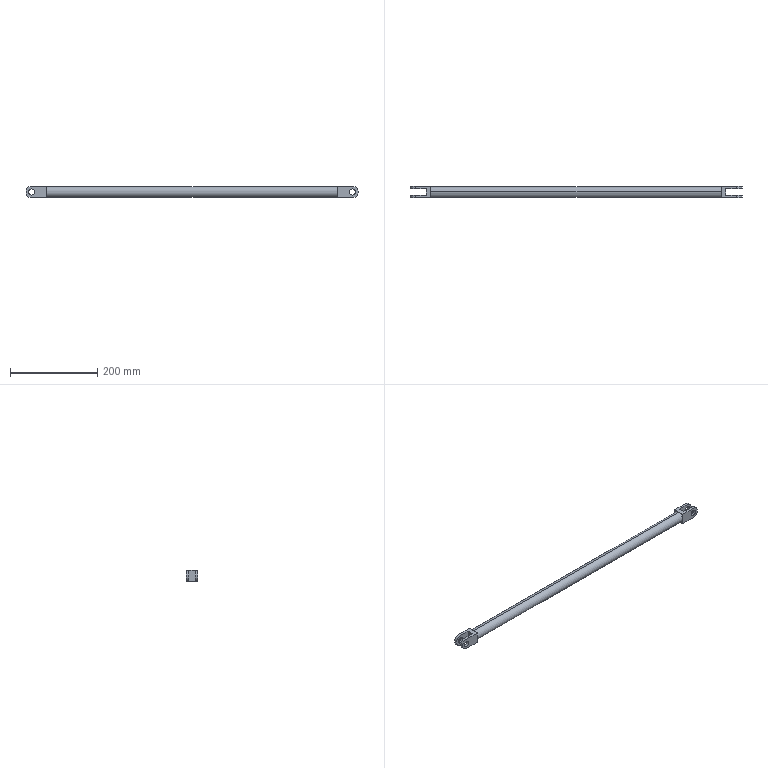Part | SolidWorks | features MirrorStock 1 | 3 solids | 34 faces | box 763 x 26 x 26 mm | volume 170096 mm3 | plane 18 | cylinder 16 | commonest cylinder face diameters 14 x8 26 x4 19 x2 25 x2
STEP:
#1=CARTESIAN_POINT('',(0.,13.,-7.));
#2=VERTEX_POINT('',#1);
#3=CARTESIAN_POINT('',(0.,13.,7.));
#4=VERTEX_POINT('',#3);
#5=CARTESIAN_POINT('',(0.,13.,0.));
#6=DIRECTION('',(0.,-1.,0.));
#7=DIRECTION('',(0.,0.,-1.));
#8=AXIS2_PLACEMENT_3D('',#5,#6,#7);
#9=CIRCLE('',#8,7.);
#10=EDGE_CURVE('',#2,#4,#9,.T.);
#11=ORIENTED_EDGE('',*,*,#10,.F.);
#12=CARTESIAN_POINT('',(0.,7.,-7.));
#13=VERTEX_POINT('',#12);
#14=CARTESIAN_POINT('',(0.,13.,-7.));
#15=DIRECTION('',(0.,-1.,0.));
#16=VECTOR('',#15,1000.);
#17=LINE('',#14,#16);
#18=EDGE_CURVE('',#2,#13,#17,.T.);
#19=ORIENTED_EDGE('',*,*,#18,.T.);
#20=CARTESIAN_POINT('',(0.,7.,7.));
#21=VERTEX_POINT('',#20);
#22=CARTESIAN_POINT('',(0.,7.,0.));
#23=DIRECTION('',(0.,-1.,0.));
#24=DIRECTION('',(-1.,0.,0.));
#25=AXIS2_PLACEMENT_3D('',#22,#23,#24);
#26=CIRCLE('',#25,7.);
#27=EDGE_CURVE('',#13,#21,#26,.T.);
#28=ORIENTED_EDGE('',*,*,#27,.T.);
#29=CARTESIAN_POINT('',(0.,13.,7.));
#30=DIRECTION('',(0.,-1.,0.));
#31=VECTOR('',#30,1000.);
#32=LINE('',#29,#31);
#33=EDGE_CURVE('',#4,#21,#32,.T.);
#34=ORIENTED_EDGE('',*,*,#33,.F.);
#35=EDGE_LOOP('',(#11,#19,#28,#34));
#36=FACE_OUTER_BOUND('',#35,.T.);
#37=CARTESIAN_POINT('',(0.,13.,0.));
#38=DIRECTION('',(0.,-1.,0.));
#39=DIRECTION('',(0.,0.,1.));
#40=AXIS2_PLACEMENT_3D('',#37,#38,#39);
#41=CYLINDRICAL_SURFACE('',#40,7.);
#42=ADVANCED_FACE('',(#36),#41,.F.);
#43=CARTESIAN_POINT('',(0.,-7.,7.));
#44=VERTEX_POINT('',#43);
#45=CARTESIAN_POINT('',(0.,-7.,-7.));
#46=VERTEX_POINT('',#45);
#47=CARTESIAN_POINT('',(0.,-7.,0.));
#48=DIRECTION('',(0.,1.,0.));
#49=DIRECTION('',(1.,0.,0.));
#50=AXIS2_PLACEMENT_3D('',#47,#48,#49);
#51=CIRCLE('',#50,7.);
#52=EDGE_CURVE('',#44,#46,#51,.T.);
#53=ORIENTED_EDGE('',*,*,#52,.T.);
#54=CARTESIAN_POINT('',(0.,-13.,-7.));
#55=VERTEX_POINT('',#54);
#56=CARTESIAN_POINT('',(0.,13.,-7.));
#57=DIRECTION('',(0.,-1.,0.));
#58=VECTOR('',#57,1000.);
#59=LINE('',#56,#58);
#60=EDGE_CURVE('',#46,#55,#59,.T.);
#61=ORIENTED_EDGE('',*,*,#60,.T.);
#62=CARTESIAN_POINT('',(0.,-13.,7.));
#63=VERTEX_POINT('',#62);
#64=CARTESIAN_POINT('',(0.,-13.,0.));
#65=DIRECTION('',(0.,-1.,0.));
#66=DIRECTION('',(0.,0.,-1.));
#67=AXIS2_PLACEMENT_3D('',#64,#65,#66);
#68=CIRCLE('',#67,7.);
#69=EDGE_CURVE('',#55,#63,#68,.T.);
#70=ORIENTED_EDGE('',*,*,#69,.T.);
#71=CARTESIAN_POINT('',(0.,13.,7.));
#72=DIRECTION('',(0.,-1.,0.));
#73=VECTOR('',#72,1000.);
#74=LINE('',#71,#73);
#75=EDGE_CURVE('',#44,#63,#74,.T.);
#76=ORIENTED_EDGE('',*,*,#75,.F.);
#77=EDGE_LOOP('',(#53,#61,#70,#76));
#78=FACE_OUTER_BOUND('',#77,.T.);
#79=CARTESIAN_POINT('',(0.,13.,0.));
#80=DIRECTION('',(0.,-1.,0.));
#81=DIRECTION('',(0.,0.,1.));
#82=AXIS2_PLACEMENT_3D('',#79,#80,#81);
#83=CYLINDRICAL_SURFACE('',#82,7.);
#84=ADVANCED_FACE('',(#78),#83,.F.);
#85=CARTESIAN_POINT('',(0.,-7.,-13.));
#86=VERTEX_POINT('',#85);
#87=CARTESIAN_POINT('',(0.,-13.,-13.));
#88=VERTEX_POINT('',#87);
#89=CARTESIAN_POINT('',(0.,13.,-13.));
#90=DIRECTION('',(0.,-1.,0.));
#91=VECTOR('',#90,1000.);
#92=LINE('',#89,#91);
#93=EDGE_CURVE('',#86,#88,#92,.T.);
#94=ORIENTED_EDGE('',*,*,#93,.T.);
#95=CARTESIAN_POINT('',(0.,-13.,13.));
#96=VERTEX_POINT('',#95);
#97=CARTESIAN_POINT('',(0.,-13.,0.));
#98=DIRECTION('',(0.,-1.,0.));
#99=DIRECTION('',(0.,0.,-1.));
#100=AXIS2_PLACEMENT_3D('',#97,#98,#99);
#101=CIRCLE('',#100,13.);
#102=EDGE_CURVE('',#96,#88,#101,.T.);
#103=ORIENTED_EDGE('',*,*,#102,.F.);
#104=CARTESIAN_POINT('',(0.,-7.,13.));
#105=VERTEX_POINT('',#104);
#106=CARTESIAN_POINT('',(0.,13.,13.));
#107=DIRECTION('',(0.,-1.,0.));
#108=VECTOR('',#107,1000.);
#109=LINE('',#106,#108);
#110=EDGE_CURVE('',#105,#96,#109,.T.);
#111=ORIENTED_EDGE('',*,*,#110,.F.);
#112=CARTESIAN_POINT('',(0.,-7.,0.));
#113=DIRECTION('',(0.,1.,0.));
#114=DIRECTION('',(1.,0.,0.));
#115=AXIS2_PLACEMENT_3D('',#112,#113,#114);
#116=CIRCLE('',#115,13.);
#117=EDGE_CURVE('',#86,#105,#116,.T.);
#118=ORIENTED_EDGE('',*,*,#117,.F.);
#119=EDGE_LOOP('',(#94,#103,#111,#118));
#120=FACE_OUTER_BOUND('',#119,.T.);
#121=CARTESIAN_POINT('',(0.,13.,0.));
#122=DIRECTION('',(0.,-1.,0.));
#123=DIRECTION('',(0.,0.,1.));
#124=AXIS2_PLACEMENT_3D('',#121,#122,#123);
#125=CYLINDRICAL_SURFACE('',#124,13.);
#126=ADVANCED_FACE('',(#120),#125,.T.);
#127=ORIENTED_EDGE('',*,*,#60,.F.);
#128=CARTESIAN_POINT('',(0.,-7.,0.));
#129=DIRECTION('',(0.,1.,0.));
#130=DIRECTION('',(1.,0.,0.));
#131=AXIS2_PLACEMENT_3D('',#128,#129,#130);
#132=CIRCLE('',#131,7.);
#133=EDGE_CURVE('',#46,#44,#132,.T.);
#134=ORIENTED_EDGE('',*,*,#133,.T.);
#135=ORIENTED_EDGE('',*,*,#75,.T.);
#136=CARTESIAN_POINT('',(0.,-13.,0.));
#137=DIRECTION('',(0.,-1.,0.));
#138=DIRECTION('',(0.,0.,-1.));
#139=AXIS2_PLACEMENT_3D('',#136,#137,#138);
#140=CIRCLE('',#139,7.);
#141=EDGE_CURVE('',#63,#55,#140,.T.);
#142=ORIENTED_EDGE('',*,*,#141,.T.);
#143=EDGE_LOOP('',(#127,#134,#135,#142));
#144=FACE_OUTER_BOUND('',#143,.T.);
#145=CARTESIAN_POINT('',(0.,13.,0.));
#146=DIRECTION('',(0.,-1.,0.));
#147=DIRECTION('',(0.,0.,1.));
#148=AXIS2_PLACEMENT_3D('',#145,#146,#147);
#149=CYLINDRICAL_SURFACE('',#148,7.);
#150=ADVANCED_FACE('',(#144),#149,.F.);
#151=CARTESIAN_POINT('',(0.,13.,13.));
#152=VERTEX_POINT('',#151);
#153=CARTESIAN_POINT('',(0.,13.,-13.));
#154=VERTEX_POINT('',#153);
#155=CARTESIAN_POINT('',(0.,13.,0.));
#156=DIRECTION('',(0.,-1.,0.));
#157=DIRECTION('',(0.,0.,-1.));
#158=AXIS2_PLACEMENT_3D('',#155,#156,#157);
#159=CIRCLE('',#158,13.);
#160=EDGE_CURVE('',#152,#154,#159,.T.);
#161=ORIENTED_EDGE('',*,*,#160,.F.);
#162=CARTESIAN_POINT('',(35.,13.,13.));
#163=VERTEX_POINT('',#162);
#164=CARTESIAN_POINT('',(0.,13.,13.));
#165=DIRECTION('',(-1.,0.,0.));
#166=VECTOR('',#165,1000.);
#167=LINE('',#164,#166);
#168=EDGE_CURVE('',#163,#152,#167,.T.);
#169=ORIENTED_EDGE('',*,*,#168,.F.);
#170=CARTESIAN_POINT('',(35.,13.,-13.));
#171=VERTEX_POINT('',#170);
#172=CARTESIAN_POINT('',(35.,13.,13.));
#173=DIRECTION('',(0.,0.,1.));
#174=VECTOR('',#173,1000.);
#175=LINE('',#172,#174);
#176=EDGE_CURVE('',#171,#163,#175,.T.);
#177=ORIENTED_EDGE('',*,*,#176,.F.);
#178=CARTESIAN_POINT('',(0.,13.,-13.));
#179=DIRECTION('',(1.,0.,0.));
#180=VECTOR('',#179,1000.);
#181=LINE('',#178,#180);
#182=EDGE_CURVE('',#154,#171,#181,.T.);
#183=ORIENTED_EDGE('',*,*,#182,.F.);
#184=EDGE_LOOP('',(#161,#169,#177,#183));
#185=FACE_OUTER_BOUND('',#184,.T.);
#186=CARTESIAN_POINT('',(0.,13.,0.));
#187=DIRECTION('',(0.,-1.,0.));
#188=DIRECTION('',(0.,0.,-1.));
#189=AXIS2_PLACEMENT_3D('',#186,#187,#188);
#190=CIRCLE('',#189,7.);
#191=EDGE_CURVE('',#4,#2,#190,.T.);
#192=ORIENTED_EDGE('',*,*,#191,.T.);
#193=ORIENTED_EDGE('',*,*,#10,.T.);
#194=EDGE_LOOP('',(#192,#193));
#195=FACE_BOUND('',#194,.T.);
#196=CARTESIAN_POINT('',(0.,13.,0.));
#197=DIRECTION('',(0.,1.,0.));
#198=DIRECTION('',(0.,0.,-1.));
#199=AXIS2_PLACEMENT_3D('',#196,#197,#198);
#200=PLANE('',#199);
#201=ADVANCED_FACE('',(#185,#195),#200,.T.);
#202=ORIENTED_EDGE('',*,*,#102,.T.);
#203=CARTESIAN_POINT('',(35.,-13.,-13.));
#204=VERTEX_POINT('',#203);
#205=CARTESIAN_POINT('',(0.,-13.,-13.));
#206=DIRECTION('',(1.,0.,0.));
#207=VECTOR('',#206,1000.);
#208=LINE('',#205,#207);
#209=EDGE_CURVE('',#88,#204,#208,.T.);
#210=ORIENTED_EDGE('',*,*,#209,.T.);
#211=CARTESIAN_POINT('',(35.,-13.,13.));
#212=VERTEX_POINT('',#211);
#213=CARTESIAN_POINT('',(35.,-13.,13.));
#214=DIRECTION('',(0.,0.,1.));
#215=VECTOR('',#214,1000.);
#216=LINE('',#213,#215);
#217=EDGE_CURVE('',#204,#212,#216,.T.);
#218=ORIENTED_EDGE('',*,*,#217,.T.);
#219=CARTESIAN_POINT('',(0.,-13.,13.));
#220=DIRECTION('',(-1.,0.,0.));
#221=VECTOR('',#220,1000.);
#222=LINE('',#219,#221);
#223=EDGE_CURVE('',#212,#96,#222,.T.);
#224=ORIENTED_EDGE('',*,*,#223,.T.);
#225=EDGE_LOOP('',(#202,#210,#218,#224));
#226=FACE_OUTER_BOUND('',#225,.T.);
#227=ORIENTED_EDGE('',*,*,#141,.F.);
#228=ORIENTED_EDGE('',*,*,#69,.F.);
#229=EDGE_LOOP('',(#227,#228));
#230=FACE_BOUND('',#229,.T.);
#231=CARTESIAN_POINT('',(0.,-13.,0.));
#232=DIRECTION('',(0.,1.,0.));
#233=DIRECTION('',(0.,0.,-1.));
#234=AXIS2_PLACEMENT_3D('',#231,#232,#233);
#235=PLANE('',#234);
#236=ADVANCED_FACE('',(#226,#230),#235,.F.);
#237=CARTESIAN_POINT('',(0.,7.,13.));
#238=VERTEX_POINT('',#237);
#239=CARTESIAN_POINT('',(0.,13.,13.));
#240=DIRECTION('',(0.,-1.,0.));
#241=VECTOR('',#240,1000.);
#242=LINE('',#239,#241);
#243=EDGE_CURVE('',#152,#238,#242,.T.);
#244=ORIENTED_EDGE('',*,*,#243,.F.);
#245=ORIENTED_EDGE('',*,*,#160,.T.);
#246=CARTESIAN_POINT('',(0.,7.,-13.));
#247=VERTEX_POINT('',#246);
#248=CARTESIAN_POINT('',(0.,13.,-13.));
#249=DIRECTION('',(0.,-1.,0.));
#250=VECTOR('',#249,1000.);
#251=LINE('',#248,#250);
#252=EDGE_CURVE('',#154,#247,#251,.T.);
#253=ORIENTED_EDGE('',*,*,#252,.T.);
#254=CARTESIAN_POINT('',(0.,7.,0.));
#255=DIRECTION('',(0.,-1.,0.));
#256=DIRECTION('',(-1.,0.,0.));
#257=AXIS2_PLACEMENT_3D('',#254,#255,#256);
#258=CIRCLE('',#257,13.);
#259=EDGE_CURVE('',#238,#247,#258,.T.);
#260=ORIENTED_EDGE('',*,*,#259,.F.);
#261=EDGE_LOOP('',(#244,#245,#253,#260));
#262=FACE_OUTER_BOUND('',#261,.T.);
#263=CARTESIAN_POINT('',(0.,13.,0.));
#264=DIRECTION('',(0.,-1.,0.));
#265=DIRECTION('',(0.,0.,1.));
#266=AXIS2_PLACEMENT_3D('',#263,#264,#265);
#267=CYLINDRICAL_SURFACE('',#266,13.);
#268=ADVANCED_FACE('',(#262),#267,.T.);
#269=CARTESIAN_POINT('',(25.,-7.,-13.));
#270=VERTEX_POINT('',#269);
#271=CARTESIAN_POINT('',(25.,7.,-13.));
#272=VERTEX_POINT('',#271);
#273=CARTESIAN_POINT('',(25.,-7.,-13.));
#274=DIRECTION('',(0.,1.,0.));
#275=VECTOR('',#274,1000.);
#276=LINE('',#273,#275);
#277=EDGE_CURVE('',#270,#272,#276,.T.);
#278=ORIENTED_EDGE('',*,*,#277,.T.);
#279=CARTESIAN_POINT('',(-25.,7.,-13.));
#280=DIRECTION('',(-1.,0.,0.));
#281=VECTOR('',#280,1000.);
#282=LINE('',#279,#281);
#283=EDGE_CURVE('',#272,#247,#282,.T.);
#284=ORIENTED_EDGE('',*,*,#283,.T.);
#285=ORIENTED_EDGE('',*,*,#252,.F.);
#286=ORIENTED_EDGE('',*,*,#182,.T.);
#287=CARTESIAN_POINT('',(35.,13.,-13.));
#288=DIRECTION('',(0.,-1.,0.));
#289=VECTOR('',#288,1000.);
#290=LINE('',#287,#289);
#291=EDGE_CURVE('',#171,#204,#290,.T.);
#292=ORIENTED_EDGE('',*,*,#291,.T.);
#293=ORIENTED_EDGE('',*,*,#209,.F.);
#294=ORIENTED_EDGE('',*,*,#93,.F.);
#295=CARTESIAN_POINT('',(-25.,-7.,-13.));
#296=DIRECTION('',(1.,0.,0.));
#297=VECTOR('',#296,1000.);
#298=LINE('',#295,#297);
#299=EDGE_CURVE('',#86,#270,#298,.T.);
#300=ORIENTED_EDGE('',*,*,#299,.T.);
#301=EDGE_LOOP('',(#278,#284,#285,#286,#292,#293,#294,#300));
#302=FACE_OUTER_BOUND('',#301,.T.);
#303=CARTESIAN_POINT('',(0.,13.,-13.));
#304=DIRECTION('',(0.,0.,1.));
#305=DIRECTION('',(-1.,0.,0.));
#306=AXIS2_PLACEMENT_3D('',#303,#304,#305);
#307=PLANE('',#306);
#308=ADVANCED_FACE('',(#302),#307,.F.);
#309=ORIENTED_EDGE('',*,*,#217,.F.);
#310=ORIENTED_EDGE('',*,*,#291,.F.);
#311=ORIENTED_EDGE('',*,*,#176,.T.);
#312=CARTESIAN_POINT('',(35.,13.,13.));
#313=DIRECTION('',(0.,-1.,0.));
#314=VECTOR('',#313,1000.);
#315=LINE('',#312,#314);
#316=EDGE_CURVE('',#163,#212,#315,.T.);
#317=ORIENTED_EDGE('',*,*,#316,.T.);
#318=EDGE_LOOP('',(#309,#310,#311,#317));
#319=FACE_OUTER_BOUND('',#318,.T.);
#320=CARTESIAN_POINT('',(35.,13.,13.));
#321=DIRECTION('',(-1.,0.,0.));
#322=DIRECTION('',(0.,0.,-1.));
#323=AXIS2_PLACEMENT_3D('',#320,#321,#322);
#324=PLANE('',#323);
#325=ADVANCED_FACE('',(#319),#324,.F.);
#326=ORIENTED_EDGE('',*,*,#110,.T.);
#327=ORIENTED_EDGE('',*,*,#223,.F.);
#328=ORIENTED_EDGE('',*,*,#316,.F.);
#329=ORIENTED_EDGE('',*,*,#168,.T.);
#330=ORIENTED_EDGE('',*,*,#243,.T.);
#331=CARTESIAN_POINT('',(25.,7.,13.));
#332=VERTEX_POINT('',#331);
#333=CARTESIAN_POINT('',(-25.,7.,13.));
#334=DIRECTION('',(-1.,0.,0.));
#335=VECTOR('',#334,1000.);
#336=LINE('',#333,#335);
#337=EDGE_CURVE('',#332,#238,#336,.T.);
#338=ORIENTED_EDGE('',*,*,#337,.F.);
#339=CARTESIAN_POINT('',(25.,-7.,13.));
#340=VERTEX_POINT('',#339);
#341=CARTESIAN_POINT('',(25.,-7.,13.));
#342=DIRECTION('',(0.,1.,0.));
#343=VECTOR('',#342,1000.);
#344=LINE('',#341,#343);
#345=EDGE_CURVE('',#340,#332,#344,.T.);
#346=ORIENTED_EDGE('',*,*,#345,.F.);
#347=CARTESIAN_POINT('',(-25.,-7.,13.));
#348=DIRECTION('',(1.,0.,0.));
#349=VECTOR('',#348,1000.);
#350=LINE('',#347,#349);
#351=EDGE_CURVE('',#105,#340,#350,.T.);
#352=ORIENTED_EDGE('',*,*,#351,.F.);
#353=EDGE_LOOP('',(#326,#327,#328,#329,#330,#338,#346,#352));
#354=FACE_OUTER_BOUND('',#353,.T.);
#355=CARTESIAN_POINT('',(0.,13.,13.));
#356=DIRECTION('',(0.,0.,-1.));
#357=DIRECTION('',(1.,0.,0.));
#358=AXIS2_PLACEMENT_3D('',#355,#356,#357);
#359=PLANE('',#358);
#360=ADVANCED_FACE('',(#354),#359,.F.);
#361=ORIENTED_EDGE('',*,*,#18,.F.);
#362=ORIENTED_EDGE('',*,*,#191,.F.);
#363=ORIENTED_EDGE('',*,*,#33,.T.);
#364=CARTESIAN_POINT('',(0.,7.,0.));
#365=DIRECTION('',(0.,-1.,0.));
#366=DIRECTION('',(-1.,0.,0.));
#367=AXIS2_PLACEMENT_3D('',#364,#365,#366);
#368=CIRCLE('',#367,7.);
#369=EDGE_CURVE('',#21,#13,#368,.T.);
#370=ORIENTED_EDGE('',*,*,#369,.T.);
#371=EDGE_LOOP('',(#361,#362,#363,#370));
#372=FACE_OUTER_BOUND('',#371,.T.);
#373=CARTESIAN_POINT('',(0.,13.,0.));
#374=DIRECTION('',(0.,-1.,0.));
#375=DIRECTION('',(0.,0.,1.));
#376=AXIS2_PLACEMENT_3D('',#373,#374,#375);
#377=CYLINDRICAL_SURFACE('',#376,7.);
#378=ADVANCED_FACE('',(#372),#377,.F.);
#379=ORIENTED_EDGE('',*,*,#52,.F.);
#380=ORIENTED_EDGE('',*,*,#133,.F.);
#381=EDGE_LOOP('',(#379,#380));
#382=FACE_BOUND('',#381,.T.);
#383=ORIENTED_EDGE('',*,*,#299,.F.);
#384=ORIENTED_EDGE('',*,*,#117,.T.);
#385=ORIENTED_EDGE('',*,*,#351,.T.);
#386=CARTESIAN_POINT('',(25.,-7.,13.));
#387=DIRECTION('',(0.,0.,-1.));
#388=VECTOR('',#387,1000.);
#389=LINE('',#386,#388);
#390=EDGE_CURVE('',#340,#270,#389,.T.);
#391=ORIENTED_EDGE('',*,*,#390,.T.);
#392=EDGE_LOOP('',(#383,#384,#385,#391));
#393=FACE_OUTER_BOUND('',#392,.T.);
#394=CARTESIAN_POINT('',(-25.,-7.,13.));
#395=DIRECTION('',(0.,-1.,0.));
#396=DIRECTION('',(1.,0.,0.));
#397=AXIS2_PLACEMENT_3D('',#394,#395,#396);
#398=PLANE('',#397);
#399=ADVANCED_FACE('',(#382,#393),#398,.F.);
#400=ORIENTED_EDGE('',*,*,#369,.F.);
#401=ORIENTED_EDGE('',*,*,#27,.F.);
#402=EDGE_LOOP('',(#400,#401));
#403=FACE_BOUND('',#402,.T.);
#404=ORIENTED_EDGE('',*,*,#337,.T.);
#405=ORIENTED_EDGE('',*,*,#259,.T.);
#406=ORIENTED_EDGE('',*,*,#283,.F.);
#407=CARTESIAN_POINT('',(25.,7.,13.));
#408=DIRECTION('',(0.,0.,-1.));
#409=VECTOR('',#408,1000.);
#410=LINE('',#407,#409);
#411=EDGE_CURVE('',#332,#272,#410,.T.);
#412=ORIENTED_EDGE('',*,*,#411,.F.);
#413=EDGE_LOOP('',(#404,#405,#406,#412));
#414=FACE_OUTER_BOUND('',#413,.T.);
#415=CARTESIAN_POINT('',(-25.,7.,13.));
#416=DIRECTION('',(0.,1.,0.));
#417=DIRECTION('',(-1.,0.,0.));
#418=AXIS2_PLACEMENT_3D('',#415,#416,#417);
#419=PLANE('',#418);
#420=ADVANCED_FACE('',(#403,#414),#419,.F.);
#421=ORIENTED_EDGE('',*,*,#411,.T.);
#422=ORIENTED_EDGE('',*,*,#277,.F.);
#423=ORIENTED_EDGE('',*,*,#390,.F.);
#424=ORIENTED_EDGE('',*,*,#345,.T.);
#425=EDGE_LOOP('',(#421,#422,#423,#424));
#426=FACE_OUTER_BOUND('',#425,.T.);
#427=CARTESIAN_POINT('',(25.,-7.,13.));
#428=DIRECTION('',(1.,0.,0.));
#429=DIRECTION('',(0.,0.,1.));
#430=AXIS2_PLACEMENT_3D('',#427,#428,#429);
#431=PLANE('',#430);
#432=ADVANCED_FACE('',(#426),#431,.F.);
#433=CLOSED_SHELL('',(#42,#84,#126,#150,#201,#236,#268,#308,#325,#360,#378,#399,#420,#432));
#434=MANIFOLD_SOLID_BREP('',#433);
#435=CARTESIAN_POINT('',(702.,0.,9.5));
#436=VERTEX_POINT('',#435);
#437=CARTESIAN_POINT('',(702.,0.,-9.5));
#438=VERTEX_POINT('',#437);
#439=CARTESIAN_POINT('',(702.,0.,0.));
#440=DIRECTION('',(-1.,0.,0.));
#441=DIRECTION('',(0.,0.,1.));
#442=AXIS2_PLACEMENT_3D('',#439,#440,#441);
#443=CIRCLE('',#442,9.5);
#444=EDGE_CURVE('',#436,#438,#443,.T.);
#445=ORIENTED_EDGE('',*,*,#444,.F.);
#446=CARTESIAN_POINT('',(35.,0.,9.5));
#447=VERTEX_POINT('',#446);
#448=CARTESIAN_POINT('',(702.,0.,9.5));
#449=DIRECTION('',(-1.,0.,0.));
#450=VECTOR('',#449,1000.);
#451=LINE('',#448,#450);
#452=EDGE_CURVE('',#436,#447,#451,.T.);
#453=ORIENTED_EDGE('',*,*,#452,.T.);
#454=CARTESIAN_POINT('',(35.,0.,-9.5));
#455=VERTEX_POINT('',#454);
#456=CARTESIAN_POINT('',(35.,0.,0.));
#457=DIRECTION('',(-1.,0.,0.));
#458=DIRECTION('',(0.,0.,1.));
#459=AXIS2_PLACEMENT_3D('',#456,#457,#458);
#460=CIRCLE('',#459,9.5);
#461=EDGE_CURVE('',#447,#455,#460,.T.);
#462=ORIENTED_EDGE('',*,*,#461,.T.);
#463=CARTESIAN_POINT('',(702.,0.,-9.5));
#464=DIRECTION('',(-1.,0.,0.));
#465=VECTOR('',#464,1000.);
#466=LINE('',#463,#465);
#467=EDGE_CURVE('',#438,#455,#466,.T.);
#468=ORIENTED_EDGE('',*,*,#467,.F.);
#469=EDGE_LOOP('',(#445,#453,#462,#468));
#470=FACE_OUTER_BOUND('',#469,.T.);
#471=CARTESIAN_POINT('',(702.,0.,0.));
#472=DIRECTION('',(-1.,0.,0.));
#473=DIRECTION('',(0.,0.,-1.));
#474=AXIS2_PLACEMENT_3D('',#471,#472,#473);
#475=CYLINDRICAL_SURFACE('',#474,9.5);
#476=ADVANCED_FACE('',(#470),#475,.F.);
#477=CARTESIAN_POINT('',(702.,0.,-12.5));
#478=VERTEX_POINT('',#477);
#479=CARTESIAN_POINT('',(702.,0.,12.5));
#480=VERTEX_POINT('',#479);
#481=CARTESIAN_POINT('',(702.,0.,0.));
#482=DIRECTION('',(-1.,0.,0.));
#483=DIRECTION('',(0.,0.,1.));
#484=AXIS2_PLACEMENT_3D('',#481,#482,#483);
#485=CIRCLE('',#484,12.5);
#486=EDGE_CURVE('',#478,#480,#485,.T.);
#487=ORIENTED_EDGE('',*,*,#486,.T.);
#488=CARTESIAN_POINT('',(35.,0.,12.5));
#489=VERTEX_POINT('',#488);
#490=CARTESIAN_POINT('',(702.,0.,12.5));
#491=DIRECTION('',(-1.,0.,0.));
#492=VECTOR('',#491,1000.);
#493=LINE('',#490,#492);
#494=EDGE_CURVE('',#480,#489,#493,.T.);
#495=ORIENTED_EDGE('',*,*,#494,.T.);
#496=CARTESIAN_POINT('',(35.,0.,-12.5));
#497=VERTEX_POINT('',#496);
#498=CARTESIAN_POINT('',(35.,0.,0.));
#499=DIRECTION('',(-1.,0.,0.));
#500=DIRECTION('',(0.,0.,1.));
#501=AXIS2_PLACEMENT_3D('',#498,#499,#500);
#502=CIRCLE('',#501,12.5);
#503=EDGE_CURVE('',#497,#489,#502,.T.);
#504=ORIENTED_EDGE('',*,*,#503,.F.);
#505=CARTESIAN_POINT('',(702.,0.,-12.5));
#506=DIRECTION('',(-1.,0.,0.));
#507=VECTOR('',#506,1000.);
#508=LINE('',#505,#507);
#509=EDGE_CURVE('',#478,#497,#508,.T.);
#510=ORIENTED_EDGE('',*,*,#509,.F.);
#511=EDGE_LOOP('',(#487,#495,#504,#510));
#512=FACE_OUTER_BOUND('',#511,.T.);
#513=CARTESIAN_POINT('',(702.,0.,0.));
#514=DIRECTION('',(-1.,0.,0.));
#515=DIRECTION('',(0.,0.,-1.));
#516=AXIS2_PLACEMENT_3D('',#513,#514,#515);
#517=CYLINDRICAL_SURFACE('',#516,12.5);
#518=ADVANCED_FACE('',(#512),#517,.T.);
#519=ORIENTED_EDGE('',*,*,#486,.F.);
#520=CARTESIAN_POINT('',(702.,0.,0.));
#521=DIRECTION('',(-1.,0.,0.));
#522=DIRECTION('',(0.,0.,1.));
#523=AXIS2_PLACEMENT_3D('',#520,#521,#522);
#524=CIRCLE('',#523,12.5);
#525=EDGE_CURVE('',#480,#478,#524,.T.);
#526=ORIENTED_EDGE('',*,*,#525,.F.);
#527=EDGE_LOOP('',(#519,#526));
#528=FACE_OUTER_BOUND('',#527,.T.);
#529=CARTESIAN_POINT('',(702.,0.,0.));
#530=DIRECTION('',(-1.,0.,0.));
#531=DIRECTION('',(0.,0.,1.));
#532=AXIS2_PLACEMENT_3D('',#529,#530,#531);
#533=CIRCLE('',#532,9.5);
#534=EDGE_CURVE('',#438,#436,#533,.T.);
#535=ORIENTED_EDGE('',*,*,#534,.T.);
#536=ORIENTED_EDGE('',*,*,#444,.T.);
#537=EDGE_LOOP('',(#535,#536));
#538=FACE_BOUND('',#537,.T.);
#539=CARTESIAN_POINT('',(702.,0.,0.));
#540=DIRECTION('',(1.,0.,0.));
#541=DIRECTION('',(0.,0.,1.));
#542=AXIS2_PLACEMENT_3D('',#539,#540,#541);
#543=PLANE('',#542);
#544=ADVANCED_FACE('',(#528,#538),#543,.T.);
#545=ORIENTED_EDGE('',*,*,#503,.T.);
#546=CARTESIAN_POINT('',(35.,0.,0.));
#547=DIRECTION('',(-1.,0.,0.));
#548=DIRECTION('',(0.,0.,1.));
#549=AXIS2_PLACEMENT_3D('',#546,#547,#548);
#550=CIRCLE('',#549,12.5);
#551=EDGE_CURVE('',#489,#497,#550,.T.);
#552=ORIENTED_EDGE('',*,*,#551,.T.);
#553=EDGE_LOOP('',(#545,#552));
#554=FACE_OUTER_BOUND('',#553,.T.);
#555=CARTESIAN_POINT('',(35.,0.,0.));
#556=DIRECTION('',(-1.,0.,0.));
#557=DIRECTION('',(0.,0.,1.));
#558=AXIS2_PLACEMENT_3D('',#555,#556,#557);
#559=CIRCLE('',#558,9.5);
#560=EDGE_CURVE('',#455,#447,#559,.T.);
#561=ORIENTED_EDGE('',*,*,#560,.F.);
#562=ORIENTED_EDGE('',*,*,#461,.F.);
#563=EDGE_LOOP('',(#561,#562));
#564=FACE_BOUND('',#563,.T.);
#565=CARTESIAN_POINT('',(35.,0.,0.));
#566=DIRECTION('',(1.,0.,0.));
#567=DIRECTION('',(0.,0.,1.));
#568=AXIS2_PLACEMENT_3D('',#565,#566,#567);
#569=PLANE('',#568);
#570=ADVANCED_FACE('',(#554,#564),#569,.F.);
#571=ORIENTED_EDGE('',*,*,#494,.F.);
#572=ORIENTED_EDGE('',*,*,#525,.T.);
#573=ORIENTED_EDGE('',*,*,#509,.T.);
#574=ORIENTED_EDGE('',*,*,#551,.F.);
#575=EDGE_LOOP('',(#571,#572,#573,#574));
#576=FACE_OUTER_BOUND('',#575,.T.);
#577=CARTESIAN_POINT('',(702.,0.,0.));
#578=DIRECTION('',(-1.,0.,0.));
#579=DIRECTION('',(0.,0.,-1.));
#580=AXIS2_PLACEMENT_3D('',#577,#578,#579);
#581=CYLINDRICAL_SURFACE('',#580,12.5);
#582=ADVANCED_FACE('',(#576),#581,.T.);
#583=ORIENTED_EDGE('',*,*,#452,.F.);
#584=ORIENTED_EDGE('',*,*,#534,.F.);
#585=ORIENTED_EDGE('',*,*,#467,.T.);
#586=ORIENTED_EDGE('',*,*,#560,.T.);
#587=EDGE_LOOP('',(#583,#584,#585,#586));
#588=FACE_OUTER_BOUND('',#587,.T.);
#589=CARTESIAN_POINT('',(702.,0.,0.));
#590=DIRECTION('',(-1.,0.,0.));
#591=DIRECTION('',(0.,0.,-1.));
#592=AXIS2_PLACEMENT_3D('',#589,#590,#591);
#593=CYLINDRICAL_SURFACE('',#592,9.5);
#594=ADVANCED_FACE('',(#588),#593,.F.);
#595=CLOSED_SHELL('',(#476,#518,#544,#570,#582,#594));
#596=MANIFOLD_SOLID_BREP('',#595);
#597=CARTESIAN_POINT('',(737.,13.,7.));
#598=VERTEX_POINT('',#597);
#599=CARTESIAN_POINT('',(737.,13.,-7.));
#600=VERTEX_POINT('',#599);
#601=CARTESIAN_POINT('',(737.,13.,0.));
#602=DIRECTION('',(0.,1.,0.));
#603=DIRECTION('',(0.,0.,-1.));
#604=AXIS2_PLACEMENT_3D('',#601,#602,#603);
#605=CIRCLE('',#604,7.);
#606=EDGE_CURVE('',#598,#600,#605,.T.);
#607=ORIENTED_EDGE('',*,*,#606,.T.);
#608=CARTESIAN_POINT('',(737.,7.,-7.));
#609=VERTEX_POINT('',#608);
#610=CARTESIAN_POINT('',(737.,13.,-7.));
#611=DIRECTION('',(0.,-1.,0.));
#612=VECTOR('',#611,1000.);
#613=LINE('',#610,#612);
#614=EDGE_CURVE('',#600,#609,#613,.T.);
#615=ORIENTED_EDGE('',*,*,#614,.T.);
#616=CARTESIAN_POINT('',(737.,7.,7.));
#617=VERTEX_POINT('',#616);
#618=CARTESIAN_POINT('',(737.,7.,0.));
#619=DIRECTION('',(0.,1.,0.));
#620=DIRECTION('',(1.,0.,0.));
#621=AXIS2_PLACEMENT_3D('',#618,#619,#620);
#622=CIRCLE('',#621,7.);
#623=EDGE_CURVE('',#617,#609,#622,.T.);
#624=ORIENTED_EDGE('',*,*,#623,.F.);
#625=CARTESIAN_POINT('',(737.,13.,7.));
#626=DIRECTION('',(0.,-1.,0.));
#627=VECTOR('',#626,1000.);
#628=LINE('',#625,#627);
#629=EDGE_CURVE('',#598,#617,#628,.T.);
#630=ORIENTED_EDGE('',*,*,#629,.F.);
#631=EDGE_LOOP('',(#607,#615,#624,#630));
#632=FACE_OUTER_BOUND('',#631,.T.);
#633=CARTESIAN_POINT('',(737.,13.,0.));
#634=DIRECTION('',(0.,-1.,0.));
#635=DIRECTION('',(0.,0.,1.));
#636=AXIS2_PLACEMENT_3D('',#633,#634,#635);
#637=CYLINDRICAL_SURFACE('',#636,7.);
#638=ADVANCED_FACE('',(#632),#637,.F.);
#639=CARTESIAN_POINT('',(737.,-7.,-7.));
#640=VERTEX_POINT('',#639);
#641=CARTESIAN_POINT('',(737.,-7.,7.));
#642=VERTEX_POINT('',#641);
#643=CARTESIAN_POINT('',(737.,-7.,0.));
#644=DIRECTION('',(0.,-1.,0.));
#645=DIRECTION('',(-1.,0.,0.));
#646=AXIS2_PLACEMENT_3D('',#643,#644,#645);
#647=CIRCLE('',#646,7.);
#648=EDGE_CURVE('',#640,#642,#647,.T.);
#649=ORIENTED_EDGE('',*,*,#648,.F.);
#650=CARTESIAN_POINT('',(737.,-13.,-7.));
#651=VERTEX_POINT('',#650);
#652=CARTESIAN_POINT('',(737.,13.,-7.));
#653=DIRECTION('',(0.,-1.,0.));
#654=VECTOR('',#653,1000.);
#655=LINE('',#652,#654);
#656=EDGE_CURVE('',#640,#651,#655,.T.);
#657=ORIENTED_EDGE('',*,*,#656,.T.);
#658=CARTESIAN_POINT('',(737.,-13.,7.));
#659=VERTEX_POINT('',#658);
#660=CARTESIAN_POINT('',(737.,-13.,0.));
#661=DIRECTION('',(0.,1.,0.));
#662=DIRECTION('',(0.,0.,-1.));
#663=AXIS2_PLACEMENT_3D('',#660,#661,#662);
#664=CIRCLE('',#663,7.);
#665=EDGE_CURVE('',#659,#651,#664,.T.);
#666=ORIENTED_EDGE('',*,*,#665,.F.);
#667=CARTESIAN_POINT('',(737.,13.,7.));
#668=DIRECTION('',(0.,-1.,0.));
#669=VECTOR('',#668,1000.);
#670=LINE('',#667,#669);
#671=EDGE_CURVE('',#642,#659,#670,.T.);
#672=ORIENTED_EDGE('',*,*,#671,.F.);
#673=EDGE_LOOP('',(#649,#657,#666,#672));
#674=FACE_OUTER_BOUND('',#673,.T.);
#675=CARTESIAN_POINT('',(737.,13.,0.));
#676=DIRECTION('',(0.,-1.,0.));
#677=DIRECTION('',(0.,0.,1.));
#678=AXIS2_PLACEMENT_3D('',#675,#676,#677);
#679=CYLINDRICAL_SURFACE('',#678,7.);
#680=ADVANCED_FACE('',(#674),#679,.F.);
#681=CARTESIAN_POINT('',(737.,-7.,-13.));
#682=VERTEX_POINT('',#681);
#683=CARTESIAN_POINT('',(737.,-13.,-13.));
#684=VERTEX_POINT('',#683);
#685=CARTESIAN_POINT('',(737.,13.,-13.));
#686=DIRECTION('',(0.,-1.,0.));
#687=VECTOR('',#686,1000.);
#688=LINE('',#685,#687);
#689=EDGE_CURVE('',#682,#684,#688,.T.);
#690=ORIENTED_EDGE('',*,*,#689,.F.);
#691=CARTESIAN_POINT('',(737.,-7.,13.));
#692=VERTEX_POINT('',#691);
#693=CARTESIAN_POINT('',(737.,-7.,0.));
#694=DIRECTION('',(0.,-1.,0.));
#695=DIRECTION('',(-1.,0.,0.));
#696=AXIS2_PLACEMENT_3D('',#693,#694,#695);
#697=CIRCLE('',#696,13.);
#698=EDGE_CURVE('',#682,#692,#697,.T.);
#699=ORIENTED_EDGE('',*,*,#698,.T.);
#700=CARTESIAN_POINT('',(737.,-13.,13.));
#701=VERTEX_POINT('',#700);
#702=CARTESIAN_POINT('',(737.,13.,13.));
#703=DIRECTION('',(0.,-1.,0.));
#704=VECTOR('',#703,1000.);
#705=LINE('',#702,#704);
#706=EDGE_CURVE('',#692,#701,#705,.T.);
#707=ORIENTED_EDGE('',*,*,#706,.T.);
#708=CARTESIAN_POINT('',(737.,-13.,0.));
#709=DIRECTION('',(0.,1.,0.));
#710=DIRECTION('',(0.,0.,-1.));
#711=AXIS2_PLACEMENT_3D('',#708,#709,#710);
#712=CIRCLE('',#711,13.);
#713=EDGE_CURVE('',#701,#684,#712,.T.);
#714=ORIENTED_EDGE('',*,*,#713,.T.);
#715=EDGE_LOOP('',(#690,#699,#707,#714));
#716=FACE_OUTER_BOUND('',#715,.T.);
#717=CARTESIAN_POINT('',(737.,13.,0.));
#718=DIRECTION('',(0.,-1.,0.));
#719=DIRECTION('',(0.,0.,1.));
#720=AXIS2_PLACEMENT_3D('',#717,#718,#719);
#721=CYLINDRICAL_SURFACE('',#720,13.);
#722=ADVANCED_FACE('',(#716),#721,.T.);
#723=ORIENTED_EDGE('',*,*,#656,.F.);
#724=CARTESIAN_POINT('',(737.,-7.,0.));
#725=DIRECTION('',(0.,-1.,0.));
#726=DIRECTION('',(-1.,0.,0.));
#727=AXIS2_PLACEMENT_3D('',#724,#725,#726);
#728=CIRCLE('',#727,7.);
#729=EDGE_CURVE('',#642,#640,#728,.T.);
#730=ORIENTED_EDGE('',*,*,#729,.F.);
#731=ORIENTED_EDGE('',*,*,#671,.T.);
#732=CARTESIAN_POINT('',(737.,-13.,0.));
#733=DIRECTION('',(0.,1.,0.));
#734=DIRECTION('',(0.,0.,-1.));
#735=AXIS2_PLACEMENT_3D('',#732,#733,#734);
#736=CIRCLE('',#735,7.);
#737=EDGE_CURVE('',#651,#659,#736,.T.);
#738=ORIENTED_EDGE('',*,*,#737,.F.);
#739=EDGE_LOOP('',(#723,#730,#731,#738));
#740=FACE_OUTER_BOUND('',#739,.T.);
#741=CARTESIAN_POINT('',(737.,13.,0.));
#742=DIRECTION('',(0.,-1.,0.));
#743=DIRECTION('',(0.,0.,1.));
#744=AXIS2_PLACEMENT_3D('',#741,#742,#743);
#745=CYLINDRICAL_SURFACE('',#744,7.);
#746=ADVANCED_FACE('',(#740),#745,.F.);
#747=CARTESIAN_POINT('',(737.,13.,13.));
#748=VERTEX_POINT('',#747);
#749=CARTESIAN_POINT('',(737.,13.,-13.));
#750=VERTEX_POINT('',#749);
#751=CARTESIAN_POINT('',(737.,13.,0.));
#752=DIRECTION('',(0.,1.,0.));
#753=DIRECTION('',(0.,0.,-1.));
#754=AXIS2_PLACEMENT_3D('',#751,#752,#753);
#755=CIRCLE('',#754,13.);
#756=EDGE_CURVE('',#748,#750,#755,.T.);
#757=ORIENTED_EDGE('',*,*,#756,.T.);
#758=CARTESIAN_POINT('',(702.,13.,-13.));
#759=VERTEX_POINT('',#758);
#760=CARTESIAN_POINT('',(737.,13.,-13.));
#761=DIRECTION('',(-1.,0.,0.));
#762=VECTOR('',#761,1000.);
#763=LINE('',#760,#762);
#764=EDGE_CURVE('',#750,#759,#763,.T.);
#765=ORIENTED_EDGE('',*,*,#764,.T.);
#766=CARTESIAN_POINT('',(702.,13.,13.));
#767=VERTEX_POINT('',#766);
#768=CARTESIAN_POINT('',(702.,13.,13.));
#769=DIRECTION('',(0.,0.,1.));
#770=VECTOR('',#769,1000.);
#771=LINE('',#768,#770);
#772=EDGE_CURVE('',#759,#767,#771,.T.);
#773=ORIENTED_EDGE('',*,*,#772,.T.);
#774=CARTESIAN_POINT('',(737.,13.,13.));
#775=DIRECTION('',(1.,0.,0.));
#776=VECTOR('',#775,1000.);
#777=LINE('',#774,#776);
#778=EDGE_CURVE('',#767,#748,#777,.T.);
#779=ORIENTED_EDGE('',*,*,#778,.T.);
#780=EDGE_LOOP('',(#757,#765,#773,#779));
#781=FACE_OUTER_BOUND('',#780,.T.);
#782=ORIENTED_EDGE('',*,*,#606,.F.);
#783=CARTESIAN_POINT('',(737.,13.,0.));
#784=DIRECTION('',(0.,1.,0.));
#785=DIRECTION('',(0.,0.,-1.));
#786=AXIS2_PLACEMENT_3D('',#783,#784,#785);
#787=CIRCLE('',#786,7.);
#788=EDGE_CURVE('',#600,#598,#787,.T.);
#789=ORIENTED_EDGE('',*,*,#788,.F.);
#790=EDGE_LOOP('',(#782,#789));
#791=FACE_BOUND('',#790,.T.);
#792=CARTESIAN_POINT('',(737.,13.,0.));
#793=DIRECTION('',(0.,1.,0.));
#794=DIRECTION('',(0.,0.,-1.));
#795=AXIS2_PLACEMENT_3D('',#792,#793,#794);
#796=PLANE('',#795);
#797=ADVANCED_FACE('',(#781,#791),#796,.T.);
#798=ORIENTED_EDGE('',*,*,#713,.F.);
#799=CARTESIAN_POINT('',(702.,-13.,13.));
#800=VERTEX_POINT('',#799);
#801=CARTESIAN_POINT('',(737.,-13.,13.));
#802=DIRECTION('',(1.,0.,0.));
#803=VECTOR('',#802,1000.);
#804=LINE('',#801,#803);
#805=EDGE_CURVE('',#800,#701,#804,.T.);
#806=ORIENTED_EDGE('',*,*,#805,.F.);
#807=CARTESIAN_POINT('',(702.,-13.,-13.));
#808=VERTEX_POINT('',#807);
#809=CARTESIAN_POINT('',(702.,-13.,13.));
#810=DIRECTION('',(0.,0.,1.));
#811=VECTOR('',#810,1000.);
#812=LINE('',#809,#811);
#813=EDGE_CURVE('',#808,#800,#812,.T.);
#814=ORIENTED_EDGE('',*,*,#813,.F.);
#815=CARTESIAN_POINT('',(737.,-13.,-13.));
#816=DIRECTION('',(-1.,0.,0.));
#817=VECTOR('',#816,1000.);
#818=LINE('',#815,#817);
#819=EDGE_CURVE('',#684,#808,#818,.T.);
#820=ORIENTED_EDGE('',*,*,#819,.F.);
#821=EDGE_LOOP('',(#798,#806,#814,#820));
#822=FACE_OUTER_BOUND('',#821,.T.);
#823=ORIENTED_EDGE('',*,*,#665,.T.);
#824=ORIENTED_EDGE('',*,*,#737,.T.);
#825=EDGE_LOOP('',(#823,#824));
#826=FACE_BOUND('',#825,.T.);
#827=CARTESIAN_POINT('',(737.,-13.,0.));
#828=DIRECTION('',(0.,1.,0.));
#829=DIRECTION('',(0.,0.,-1.));
#830=AXIS2_PLACEMENT_3D('',#827,#828,#829);
#831=PLANE('',#830);
#832=ADVANCED_FACE('',(#822,#826),#831,.F.);
#833=CARTESIAN_POINT('',(737.,7.,13.));
#834=VERTEX_POINT('',#833);
#835=CARTESIAN_POINT('',(737.,13.,13.));
#836=DIRECTION('',(0.,-1.,0.));
#837=VECTOR('',#836,1000.);
#838=LINE('',#835,#837);
#839=EDGE_CURVE('',#748,#834,#838,.T.);
#840=ORIENTED_EDGE('',*,*,#839,.T.);
#841=CARTESIAN_POINT('',(737.,7.,-13.));
#842=VERTEX_POINT('',#841);
#843=CARTESIAN_POINT('',(737.,7.,0.));
#844=DIRECTION('',(0.,1.,0.));
#845=DIRECTION('',(1.,0.,0.));
#846=AXIS2_PLACEMENT_3D('',#843,#844,#845);
#847=CIRCLE('',#846,13.);
#848=EDGE_CURVE('',#834,#842,#847,.T.);
#849=ORIENTED_EDGE('',*,*,#848,.T.);
#850=CARTESIAN_POINT('',(737.,13.,-13.));
#851=DIRECTION('',(0.,-1.,0.));
#852=VECTOR('',#851,1000.);
#853=LINE('',#850,#852);
#854=EDGE_CURVE('',#750,#842,#853,.T.);
#855=ORIENTED_EDGE('',*,*,#854,.F.);
#856=ORIENTED_EDGE('',*,*,#756,.F.);
#857=EDGE_LOOP('',(#840,#849,#855,#856));
#858=FACE_OUTER_BOUND('',#857,.T.);
#859=CARTESIAN_POINT('',(737.,13.,0.));
#860=DIRECTION('',(0.,-1.,0.));
#861=DIRECTION('',(0.,0.,1.));
#862=AXIS2_PLACEMENT_3D('',#859,#860,#861);
#863=CYLINDRICAL_SURFACE('',#862,13.);
#864=ADVANCED_FACE('',(#858),#863,.T.);
#865=CARTESIAN_POINT('',(712.,-7.,-13.));
#866=VERTEX_POINT('',#865);
#867=CARTESIAN_POINT('',(712.,7.,-13.));
#868=VERTEX_POINT('',#867);
#869=CARTESIAN_POINT('',(712.,-7.,-13.));
#870=DIRECTION('',(0.,1.,0.));
#871=VECTOR('',#870,1000.);
#872=LINE('',#869,#871);
#873=EDGE_CURVE('',#866,#868,#872,.T.);
#874=ORIENTED_EDGE('',*,*,#873,.F.);
#875=CARTESIAN_POINT('',(762.,-7.,-13.));
#876=DIRECTION('',(-1.,0.,0.));
#877=VECTOR('',#876,1000.);
#878=LINE('',#875,#877);
#879=EDGE_CURVE('',#682,#866,#878,.T.);
#880=ORIENTED_EDGE('',*,*,#879,.F.);
#881=ORIENTED_EDGE('',*,*,#689,.T.);
#882=ORIENTED_EDGE('',*,*,#819,.T.);
#883=CARTESIAN_POINT('',(702.,13.,-13.));
#884=DIRECTION('',(0.,-1.,0.));
#885=VECTOR('',#884,1000.);
#886=LINE('',#883,#885);
#887=EDGE_CURVE('',#759,#808,#886,.T.);
#888=ORIENTED_EDGE('',*,*,#887,.F.);
#889=ORIENTED_EDGE('',*,*,#764,.F.);
#890=ORIENTED_EDGE('',*,*,#854,.T.);
#891=CARTESIAN_POINT('',(762.,7.,-13.));
#892=DIRECTION('',(1.,0.,0.));
#893=VECTOR('',#892,1000.);
#894=LINE('',#891,#893);
#895=EDGE_CURVE('',#868,#842,#894,.T.);
#896=ORIENTED_EDGE('',*,*,#895,.F.);
#897=EDGE_LOOP('',(#874,#880,#881,#882,#888,#889,#890,#896));
#898=FACE_OUTER_BOUND('',#897,.T.);
#899=CARTESIAN_POINT('',(737.,13.,-13.));
#900=DIRECTION('',(0.,0.,1.));
#901=DIRECTION('',(1.,0.,0.));
#902=AXIS2_PLACEMENT_3D('',#899,#900,#901);
#903=PLANE('',#902);
#904=ADVANCED_FACE('',(#898),#903,.F.);
#905=ORIENTED_EDGE('',*,*,#813,.T.);
#906=CARTESIAN_POINT('',(702.,13.,13.));
#907=DIRECTION('',(0.,-1.,0.));
#908=VECTOR('',#907,1000.);
#909=LINE('',#906,#908);
#910=EDGE_CURVE('',#767,#800,#909,.T.);
#911=ORIENTED_EDGE('',*,*,#910,.F.);
#912=ORIENTED_EDGE('',*,*,#772,.F.);
#913=ORIENTED_EDGE('',*,*,#887,.T.);
#914=EDGE_LOOP('',(#905,#911,#912,#913));
#915=FACE_OUTER_BOUND('',#914,.T.);
#916=CARTESIAN_POINT('',(702.,13.,13.));
#917=DIRECTION('',(1.,0.,0.));
#918=DIRECTION('',(0.,0.,-1.));
#919=AXIS2_PLACEMENT_3D('',#916,#917,#918);
#920=PLANE('',#919);
#921=ADVANCED_FACE('',(#915),#920,.F.);
#922=ORIENTED_EDGE('',*,*,#706,.F.);
#923=CARTESIAN_POINT('',(712.,-7.,13.));
#924=VERTEX_POINT('',#923);
#925=CARTESIAN_POINT('',(762.,-7.,13.));
#926=DIRECTION('',(-1.,0.,0.));
#927=VECTOR('',#926,1000.);
#928=LINE('',#925,#927);
#929=EDGE_CURVE('',#692,#924,#928,.T.);
#930=ORIENTED_EDGE('',*,*,#929,.T.);
#931=CARTESIAN_POINT('',(712.,7.,13.));
#932=VERTEX_POINT('',#931);
#933=CARTESIAN_POINT('',(712.,-7.,13.));
#934=DIRECTION('',(0.,1.,0.));
#935=VECTOR('',#934,1000.);
#936=LINE('',#933,#935);
#937=EDGE_CURVE('',#924,#932,#936,.T.);
#938=ORIENTED_EDGE('',*,*,#937,.T.);
#939=CARTESIAN_POINT('',(762.,7.,13.));
#940=DIRECTION('',(1.,0.,0.));
#941=VECTOR('',#940,1000.);
#942=LINE('',#939,#941);
#943=EDGE_CURVE('',#932,#834,#942,.T.);
#944=ORIENTED_EDGE('',*,*,#943,.T.);
#945=ORIENTED_EDGE('',*,*,#839,.F.);
#946=ORIENTED_EDGE('',*,*,#778,.F.);
#947=ORIENTED_EDGE('',*,*,#910,.T.);
#948=ORIENTED_EDGE('',*,*,#805,.T.);
#949=EDGE_LOOP('',(#922,#930,#938,#944,#945,#946,#947,#948));
#950=FACE_OUTER_BOUND('',#949,.T.);
#951=CARTESIAN_POINT('',(737.,13.,13.));
#952=DIRECTION('',(0.,0.,-1.));
#953=DIRECTION('',(-1.,0.,0.));
#954=AXIS2_PLACEMENT_3D('',#951,#952,#953);
#955=PLANE('',#954);
#956=ADVANCED_FACE('',(#950),#955,.F.);
#957=ORIENTED_EDGE('',*,*,#614,.F.);
#958=ORIENTED_EDGE('',*,*,#788,.T.);
#959=ORIENTED_EDGE('',*,*,#629,.T.);
#960=CARTESIAN_POINT('',(737.,7.,0.));
#961=DIRECTION('',(0.,1.,0.));
#962=DIRECTION('',(1.,0.,0.));
#963=AXIS2_PLACEMENT_3D('',#960,#961,#962);
#964=CIRCLE('',#963,7.);
#965=EDGE_CURVE('',#609,#617,#964,.T.);
#966=ORIENTED_EDGE('',*,*,#965,.F.);
#967=EDGE_LOOP('',(#957,#958,#959,#966));
#968=FACE_OUTER_BOUND('',#967,.T.);
#969=CARTESIAN_POINT('',(737.,13.,0.));
#970=DIRECTION('',(0.,-1.,0.));
#971=DIRECTION('',(0.,0.,1.));
#972=AXIS2_PLACEMENT_3D('',#969,#970,#971);
#973=CYLINDRICAL_SURFACE('',#972,7.);
#974=ADVANCED_FACE('',(#968),#973,.F.);
#975=ORIENTED_EDGE('',*,*,#729,.T.);
#976=ORIENTED_EDGE('',*,*,#648,.T.);
#977=EDGE_LOOP('',(#975,#976));
#978=FACE_BOUND('',#977,.T.);
#979=ORIENTED_EDGE('',*,*,#879,.T.);
#980=CARTESIAN_POINT('',(712.,-7.,13.));
#981=DIRECTION('',(0.,0.,-1.));
#982=VECTOR('',#981,1000.);
#983=LINE('',#980,#982);
#984=EDGE_CURVE('',#924,#866,#983,.T.);
#985=ORIENTED_EDGE('',*,*,#984,.F.);
#986=ORIENTED_EDGE('',*,*,#929,.F.);
#987=ORIENTED_EDGE('',*,*,#698,.F.);
#988=EDGE_LOOP('',(#979,#985,#986,#987));
#989=FACE_OUTER_BOUND('',#988,.T.);
#990=CARTESIAN_POINT('',(762.,-7.,13.));
#991=DIRECTION('',(0.,-1.,0.));
#992=DIRECTION('',(-1.,0.,0.));
#993=AXIS2_PLACEMENT_3D('',#990,#991,#992);
#994=PLANE('',#993);
#995=ADVANCED_FACE('',(#978,#989),#994,.F.);
#996=ORIENTED_EDGE('',*,*,#623,.T.);
#997=ORIENTED_EDGE('',*,*,#965,.T.);
#998=EDGE_LOOP('',(#996,#997));
#999=FACE_BOUND('',#998,.T.);
#1000=ORIENTED_EDGE('',*,*,#943,.F.);
#1001=CARTESIAN_POINT('',(712.,7.,13.));
#1002=DIRECTION('',(0.,0.,-1.));
#1003=VECTOR('',#1002,1000.);
#1004=LINE('',#1001,#1003);
#1005=EDGE_CURVE('',#932,#868,#1004,.T.);
#1006=ORIENTED_EDGE('',*,*,#1005,.T.);
#1007=ORIENTED_EDGE('',*,*,#895,.T.);
#1008=ORIENTED_EDGE('',*,*,#848,.F.);
#1009=EDGE_LOOP('',(#1000,#1006,#1007,#1008));
#1010=FACE_OUTER_BOUND('',#1009,.T.);
#1011=CARTESIAN_POINT('',(762.,7.,13.));
#1012=DIRECTION('',(0.,1.,0.));
#1013=DIRECTION('',(1.,0.,0.));
#1014=AXIS2_PLACEMENT_3D('',#1011,#1012,#1013);
#1015=PLANE('',#1014);
#1016=ADVANCED_FACE('',(#999,#1010),#1015,.F.);
#1017=ORIENTED_EDGE('',*,*,#1005,.F.);
#1018=ORIENTED_EDGE('',*,*,#937,.F.);
#1019=ORIENTED_EDGE('',*,*,#984,.T.);
#1020=ORIENTED_EDGE('',*,*,#873,.T.);
#1021=EDGE_LOOP('',(#1017,#1018,#1019,#1020));
#1022=FACE_OUTER_BOUND('',#1021,.T.);
#1023=CARTESIAN_POINT('',(712.,-7.,13.));
#1024=DIRECTION('',(-1.,0.,0.));
#1025=DIRECTION('',(0.,0.,1.));
#1026=AXIS2_PLACEMENT_3D('',#1023,#1024,#1025);
#1027=PLANE('',#1026);
#1028=ADVANCED_FACE('',(#1022),#1027,.F.);
#1029=CLOSED_SHELL('',(#638,#680,#722,#746,#797,#832,#864,#904,#921,#956,#974,#995,#1016,#1028));
#1030=MANIFOLD_SOLID_BREP('',#1029);
#1031=CARTESIAN_POINT('',(0.,0.,0.));
#1032=DIRECTION('',(0.,0.,1.));
#1033=DIRECTION('',(1.,0.,0.));
#1034=AXIS2_PLACEMENT_3D('',#1031,#1032,#1033);
#1035=(LENGTH_UNIT()NAMED_UNIT(*)SI_UNIT(.MILLI.,.METRE.));
#1036=UNCERTAINTY_MEASURE_WITH_UNIT(LENGTH_MEASURE(0.00001),#1035,'','');
#1037=(NAMED_UNIT(*)PLANE_ANGLE_UNIT()SI_UNIT($,.RADIAN.));
#1038=(NAMED_UNIT(*)SI_UNIT($,.STERADIAN.)SOLID_ANGLE_UNIT());
#1039=(GEOMETRIC_REPRESENTATION_CONTEXT(3)GLOBAL_UNCERTAINTY_ASSIGNED_CONTEXT((#1036))GLOBAL_UNIT_ASSIGNED_CONTEXT((#1035,#1037,#1038))REPRESENTATION_CONTEXT('',''));
#1040=ADVANCED_BREP_SHAPE_REPRESENTATION('',(#434,#596,#1030,#1034),#1039);